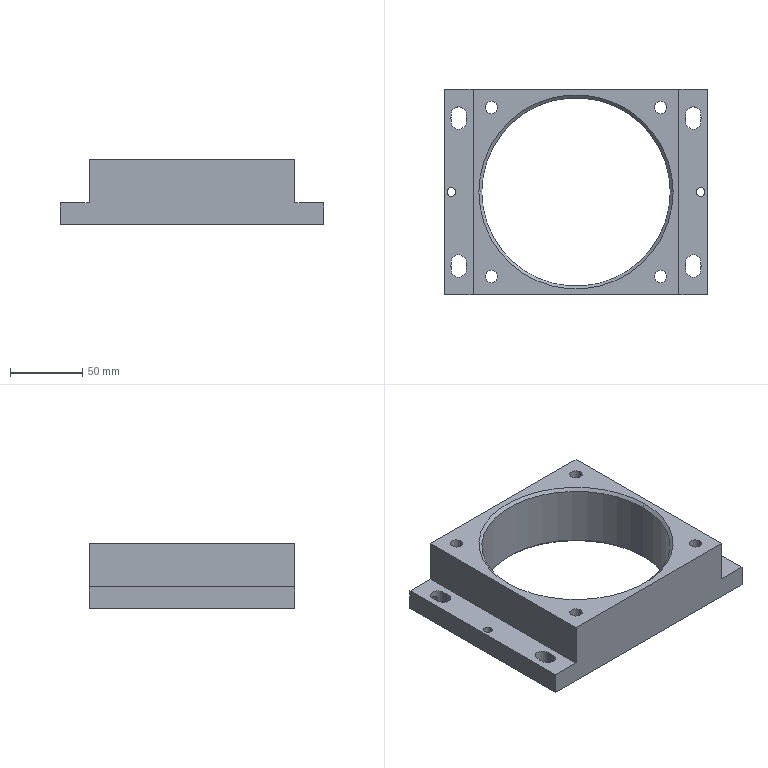CAM job | NX | 3-axis milling, drilling | part box 182 x 142 x 45 mm | stock box 182 x 142 x 45 mm
Tools:
number,name,description,diameter,corner_radius,flute_length,length,flutes
10,D10,Milling Tool-5 Parameters,10.0,0.0,50.0,75.0,2
11,D10JING,Milling Tool-5 Parameters,10.0,0.0,50.0,75.0,2
7,D6A45,Milling Tool-5 Parameters,6.0,0.0,3.0,3.0,2
6,D6,Milling Tool-5 Parameters,6.0,0.0,50.0,75.0,2
8,8.5ZT,Drilling Tool,8.5,0.0,35.0,50.0,2
16,6.0ZT,Drilling Tool,6.0,0.0,35.0,50.0,2
Operations:
program,operation,operation_type,tool,method,geometry_group,spindle_rpm,surface_speed,feed_per_tooth,feed_cut,feed_plunge,cut_length_mm,path_length_mm,cut_time_min,machine_time_min
1-45-182-142毛胚,ADAPTIVE_MILLING,CavityMilling,D10,METHOD,A,8000.0,251.0,0.2188,3500.0,1000.0,48217.275,59729.469,15.962,17.113
1-45-182-142毛胚,DRILLING_COPY_1,Operation,D6A45,METHOD,A,3000.0,56.0,0.0333,200.0,0.0,24.0,524.69,0.12,0.1701
1-45-182-142毛胚,DRILLING_COPY_1_COPY,Operation,8.5ZT,METHOD,A,2000.0,42.0,0.05,200.0,0.0,208.215,835.563,1.041,1.104
1-45-182-142毛胚,DRILLING_COPY_1_COPY_COPY,Operation,6.0ZT,METHOD,A,2000.0,42.0,0.05,200.0,0.0,42.605,380.236,0.213,0.2468
1-45-182-142毛胚,ZLEVEL_PROFILE_COPY_COPY_1,ZLevelMilling,D10JING,METHOD,A,8000.0,251.0,0.05,800.0,100.0,317.326,686.899,0.3967,0.4336
1-45-182-142毛胚,FLOOR_WALL_1_COPY_1,VolumeBased25DMillingOperation,D10JING,METHOD,A,7500.0,94.0,0.0533,800.0,100.0,1892.082,2617.056,2.365,2.458
1-45-182-142毛胚,ZLEVEL_PROFILE_COPY_1_COPY,ZLevelMilling,D6,METHOD,A,7500.0,141.0,0.12,1800.0,100.0,3084.882,3979.726,1.714,1.803
1-45-182-142毛胚,ZLEVEL_PROFILE_COPY_COPY_1_1,ZLevelMilling,D6,METHOD,A,8000.0,251.0,0.05,800.0,100.0,116.9,1075.44,0.1461,0.242
1-45-182-142毛胚,ZLEVEL_PROFILE_1_COPY_1_COPY_COPY_1_COPY,ZLevelMilling,D6A45,METHOD,A,7500.0,141.0,0.0667,1000.0,100.0,687.973,1365.165,0.688,0.7557
1-45-182-142毛胚,ZLEVEL_PROFILE_1_COPY_1_COPY_COPY_1_COPY_COPY,ZLevelMilling,D6A45,METHOD,A,7500.0,141.0,0.0667,1000.0,100.0,410.62,473.62,0.4106,0.4169
1-45-182-142毛胚,ZLEVEL_PROFILE_1_COPY_1_COPY_COPY_1_COPY_COPY_1,ZLevelMilling,D6A45,METHOD,A,7500.0,141.0,0.0667,1000.0,100.0,545.689,2571.514,0.5457,0.7483
1-45-182-142毛胚,刀补11,ZLevelMilling,D10JING,METHOD,A,8000.0,251.0,0.05,800.0,100.0,766.25,914.53,0.9578,0.9726